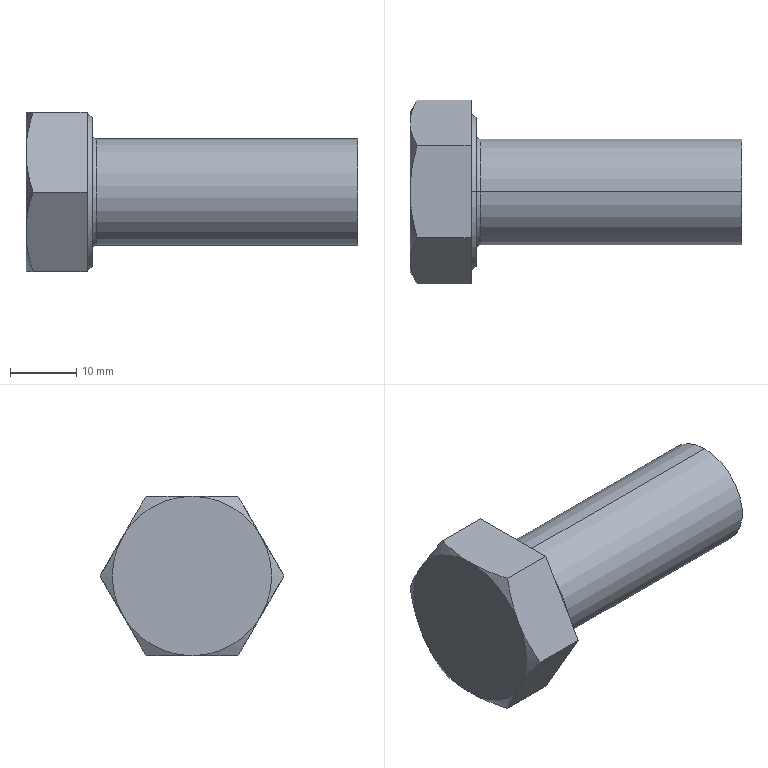Part | SolidWorks | features RevCut 3, Extrusion 1, Fillet 1, LPattern 1, Revolution 1 | 1 solid | 22 faces | box 50 x 27.713 x 24 mm | volume 12952 mm3 | plane 10 | cone 8 | torus 2 | cylinder 2 | commonest cylinder face diameters 16 x2
STEP:
#1=CARTESIAN_POINT('',(10.6,0.,8.));
#2=VERTEX_POINT('',#1);
#3=CARTESIAN_POINT('',(10.6,0.,-8.));
#4=VERTEX_POINT('',#3);
#5=CARTESIAN_POINT('',(10.6,0.,0.));
#6=DIRECTION('',(1.,0.,0.));
#7=DIRECTION('',(0.,0.,-1.));
#8=AXIS2_PLACEMENT_3D('',#5,#6,#7);
#9=CIRCLE('',#8,8.);
#10=EDGE_CURVE('',#2,#4,#9,.T.);
#11=ORIENTED_EDGE('',*,*,#10,.F.);
#12=CARTESIAN_POINT('',(10.,0.,8.6));
#13=VERTEX_POINT('',#12);
#14=CARTESIAN_POINT('',(10.6,0.,8.6));
#15=DIRECTION('',(0.,1.,0.));
#16=DIRECTION('',(0.,0.,1.));
#17=AXIS2_PLACEMENT_3D('',#14,#15,#16);
#18=CIRCLE('',#17,0.6);
#19=EDGE_CURVE('',#2,#13,#18,.T.);
#20=ORIENTED_EDGE('',*,*,#19,.T.);
#21=CARTESIAN_POINT('',(10.,0.,-8.6));
#22=VERTEX_POINT('',#21);
#23=CARTESIAN_POINT('',(10.,0.,0.));
#24=DIRECTION('',(-1.,0.,0.));
#25=DIRECTION('',(0.,0.,-1.));
#26=AXIS2_PLACEMENT_3D('',#23,#24,#25);
#27=CIRCLE('',#26,8.6);
#28=EDGE_CURVE('',#22,#13,#27,.T.);
#29=ORIENTED_EDGE('',*,*,#28,.F.);
#30=CARTESIAN_POINT('',(10.6,0.,-8.6));
#31=DIRECTION('',(0.,-1.,0.));
#32=DIRECTION('',(0.,0.,-1.));
#33=AXIS2_PLACEMENT_3D('',#30,#31,#32);
#34=CIRCLE('',#33,0.6);
#35=EDGE_CURVE('',#4,#22,#34,.T.);
#36=ORIENTED_EDGE('',*,*,#35,.F.);
#37=EDGE_LOOP('',(#11,#20,#29,#36));
#38=FACE_OUTER_BOUND('',#37,.T.);
#39=CARTESIAN_POINT('',(10.6,0.,0.));
#40=DIRECTION('',(1.,0.,0.));
#41=DIRECTION('',(0.,0.,-1.));
#42=AXIS2_PLACEMENT_3D('',#39,#40,#41);
#43=TOROIDAL_SURFACE('',#42,8.6,0.6);
#44=ADVANCED_FACE('',(#38),#43,.F.);
#45=CARTESIAN_POINT('',(50.,0.,8.));
#46=VERTEX_POINT('',#45);
#47=CARTESIAN_POINT('',(50.,0.,-8.));
#48=VERTEX_POINT('',#47);
#49=CARTESIAN_POINT('',(50.,0.,0.));
#50=DIRECTION('',(-1.,0.,0.));
#51=DIRECTION('',(0.,0.,1.));
#52=AXIS2_PLACEMENT_3D('',#49,#50,#51);
#53=CIRCLE('',#52,8.);
#54=EDGE_CURVE('',#46,#48,#53,.T.);
#55=ORIENTED_EDGE('',*,*,#54,.T.);
#56=CARTESIAN_POINT('',(0.,0.,-8.));
#57=DIRECTION('',(-1.,0.,0.));
#58=VECTOR('',#57,1000.);
#59=LINE('',#56,#58);
#60=EDGE_CURVE('',#48,#4,#59,.T.);
#61=ORIENTED_EDGE('',*,*,#60,.T.);
#62=CARTESIAN_POINT('',(10.6,0.,0.));
#63=DIRECTION('',(1.,0.,0.));
#64=DIRECTION('',(0.,0.,-1.));
#65=AXIS2_PLACEMENT_3D('',#62,#63,#64);
#66=CIRCLE('',#65,8.);
#67=EDGE_CURVE('',#4,#2,#66,.T.);
#68=ORIENTED_EDGE('',*,*,#67,.T.);
#69=CARTESIAN_POINT('',(0.,0.,8.));
#70=DIRECTION('',(-1.,0.,0.));
#71=VECTOR('',#70,1000.);
#72=LINE('',#69,#71);
#73=EDGE_CURVE('',#46,#2,#72,.T.);
#74=ORIENTED_EDGE('',*,*,#73,.F.);
#75=EDGE_LOOP('',(#55,#61,#68,#74));
#76=FACE_OUTER_BOUND('',#75,.T.);
#77=CARTESIAN_POINT('',(0.,0.,0.));
#78=DIRECTION('',(-1.,0.,0.));
#79=DIRECTION('',(0.,0.,1.));
#80=AXIS2_PLACEMENT_3D('',#77,#78,#79);
#81=CYLINDRICAL_SURFACE('',#80,8.);
#82=ADVANCED_FACE('',(#76),#81,.T.);
#83=CARTESIAN_POINT('',(10.,0.,11.245));
#84=VERTEX_POINT('',#83);
#85=CARTESIAN_POINT('',(10.,0.,-11.245));
#86=VERTEX_POINT('',#85);
#87=CARTESIAN_POINT('',(10.,0.,0.));
#88=DIRECTION('',(-1.,0.,0.));
#89=DIRECTION('',(0.,0.,1.));
#90=AXIS2_PLACEMENT_3D('',#87,#88,#89);
#91=CIRCLE('',#90,11.245);
#92=EDGE_CURVE('',#84,#86,#91,.T.);
#93=ORIENTED_EDGE('',*,*,#92,.T.);
#94=CARTESIAN_POINT('',(9.2,0.,-11.707));
#95=VERTEX_POINT('',#94);
#96=CARTESIAN_POINT('',(9.2,0.,-11.707));
#97=DIRECTION('',(-0.866,0.,-0.5));
#98=VECTOR('',#97,1000.);
#99=LINE('',#96,#98);
#100=EDGE_CURVE('',#86,#95,#99,.T.);
#101=ORIENTED_EDGE('',*,*,#100,.T.);
#102=CARTESIAN_POINT('',(9.2,0.,11.707));
#103=VERTEX_POINT('',#102);
#104=CARTESIAN_POINT('',(9.2,0.,0.));
#105=DIRECTION('',(-1.,0.,0.));
#106=DIRECTION('',(0.,0.,1.));
#107=AXIS2_PLACEMENT_3D('',#104,#105,#106);
#108=CIRCLE('',#107,11.707);
#109=EDGE_CURVE('',#103,#95,#108,.T.);
#110=ORIENTED_EDGE('',*,*,#109,.F.);
#111=CARTESIAN_POINT('',(9.2,0.,11.707));
#112=DIRECTION('',(-0.866,0.,0.5));
#113=VECTOR('',#112,1000.);
#114=LINE('',#111,#113);
#115=EDGE_CURVE('',#84,#103,#114,.T.);
#116=ORIENTED_EDGE('',*,*,#115,.F.);
#117=EDGE_LOOP('',(#93,#101,#110,#116));
#118=FACE_OUTER_BOUND('',#117,.T.);
#119=CARTESIAN_POINT('',(9.2,0.,0.));
#120=DIRECTION('',(-1.,0.,0.));
#121=DIRECTION('',(0.,0.,1.));
#122=AXIS2_PLACEMENT_3D('',#119,#120,#121);
#123=CONICAL_SURFACE('',#122,11.707,0.5236);
#124=ADVANCED_FACE('',(#118),#123,.T.);
#125=CARTESIAN_POINT('',(9.2,6.928,-12.));
#126=VERTEX_POINT('',#125);
#127=CARTESIAN_POINT('',(9.2,13.856,0.));
#128=VERTEX_POINT('',#127);
#129=CARTESIAN_POINT('',(9.2,6.928,-12.));
#130=DIRECTION('',(0.,0.5,0.866));
#131=VECTOR('',#130,1000.);
#132=LINE('',#129,#131);
#133=EDGE_CURVE('',#126,#128,#132,.T.);
#134=ORIENTED_EDGE('',*,*,#133,.F.);
#135=CARTESIAN_POINT('',(1.072,6.928,-12.));
#136=VERTEX_POINT('',#135);
#137=CARTESIAN_POINT('',(10.,6.928,-12.));
#138=DIRECTION('',(-1.,0.,0.));
#139=VECTOR('',#138,1000.);
#140=LINE('',#137,#139);
#141=EDGE_CURVE('',#126,#136,#140,.T.);
#142=ORIENTED_EDGE('',*,*,#141,.T.);
#143=CARTESIAN_POINT('',(0.,10.392,-6.));
#144=VERTEX_POINT('',#143);
#145=CARTESIAN_POINT('',(0.,10.392,-6.));
#146=CARTESIAN_POINT('',(0.,10.098,-6.509));
#147=CARTESIAN_POINT('',(0.02533,9.803,-7.021));
#148=CARTESIAN_POINT('',(0.1234,9.219,-8.033));
#149=CARTESIAN_POINT('',(0.196,8.929,-8.535));
#150=CARTESIAN_POINT('',(0.476,8.063,-10.034));
#151=CARTESIAN_POINT('',(0.7454,7.493,-11.021));
#152=CARTESIAN_POINT('',(1.072,6.928,-12.));
#153=B_SPLINE_CURVE_WITH_KNOTS('',3,(#145,#146,#147,#148,#149,#150,#151,#152),.UNSPECIFIED.,.F.,.F.,(4,2,2,4),(0.00701,0.008756,0.0105,0.01399),.UNSPECIFIED.);
#154=EDGE_CURVE('',#144,#136,#153,.T.);
#155=ORIENTED_EDGE('',*,*,#154,.F.);
#156=CARTESIAN_POINT('',(1.072,13.856,0.));
#157=VERTEX_POINT('',#156);
#158=CARTESIAN_POINT('',(1.072,13.856,0.));
#159=CARTESIAN_POINT('',(0.7446,13.29,-0.9815));
#160=CARTESIAN_POINT('',(0.4751,12.719,-1.97));
#161=CARTESIAN_POINT('',(0.1021,11.565,-3.968));
#162=CARTESIAN_POINT('',(0.,10.982,-4.978));
#163=CARTESIAN_POINT('',(0.,10.392,-6.));
#164=B_SPLINE_CURVE_WITH_KNOTS('',3,(#158,#159,#160,#161,#162,#163),.UNSPECIFIED.,.F.,.F.,(4,2,4),(0.000000238,0.003505,0.00701),.UNSPECIFIED.);
#165=EDGE_CURVE('',#157,#144,#164,.T.);
#166=ORIENTED_EDGE('',*,*,#165,.F.);
#167=CARTESIAN_POINT('',(10.,13.856,0.));
#168=DIRECTION('',(-1.,0.,0.));
#169=VECTOR('',#168,1000.);
#170=LINE('',#167,#169);
#171=EDGE_CURVE('',#128,#157,#170,.T.);
#172=ORIENTED_EDGE('',*,*,#171,.F.);
#173=EDGE_LOOP('',(#134,#142,#155,#166,#172));
#174=FACE_OUTER_BOUND('',#173,.T.);
#175=CARTESIAN_POINT('',(10.,6.928,-12.));
#176=DIRECTION('',(0.,-0.866,0.5));
#177=DIRECTION('',(0.,-0.5,-0.866));
#178=AXIS2_PLACEMENT_3D('',#175,#176,#177);
#179=PLANE('',#178);
#180=ADVANCED_FACE('',(#174),#179,.F.);
#181=CARTESIAN_POINT('',(9.2,6.928,12.));
#182=VERTEX_POINT('',#181);
#183=CARTESIAN_POINT('',(9.2,13.856,0.));
#184=DIRECTION('',(0.,-0.5,0.866));
#185=VECTOR('',#184,1000.);
#186=LINE('',#183,#185);
#187=EDGE_CURVE('',#128,#182,#186,.T.);
#188=ORIENTED_EDGE('',*,*,#187,.F.);
#189=ORIENTED_EDGE('',*,*,#171,.T.);
#190=CARTESIAN_POINT('',(0.,10.392,6.));
#191=VERTEX_POINT('',#190);
#192=CARTESIAN_POINT('',(0.,10.392,6.));
#193=CARTESIAN_POINT('',(0.,10.686,5.491));
#194=CARTESIAN_POINT('',(0.02533,10.982,4.979));
#195=CARTESIAN_POINT('',(0.1234,11.566,3.967));
#196=CARTESIAN_POINT('',(0.196,11.856,3.465));
#197=CARTESIAN_POINT('',(0.476,12.721,1.966));
#198=CARTESIAN_POINT('',(0.7454,13.291,0.9791));
#199=CARTESIAN_POINT('',(1.072,13.856,0.));
#200=B_SPLINE_CURVE_WITH_KNOTS('',3,(#192,#193,#194,#195,#196,#197,#198,#199),.UNSPECIFIED.,.F.,.F.,(4,2,2,4),(0.00701,0.008756,0.0105,0.01399),.UNSPECIFIED.);
#201=EDGE_CURVE('',#191,#157,#200,.T.);
#202=ORIENTED_EDGE('',*,*,#201,.F.);
#203=CARTESIAN_POINT('',(1.072,6.928,12.));
#204=VERTEX_POINT('',#203);
#205=CARTESIAN_POINT('',(1.072,6.928,12.));
#206=CARTESIAN_POINT('',(0.7446,7.495,11.018));
#207=CARTESIAN_POINT('',(0.4751,8.066,10.03));
#208=CARTESIAN_POINT('',(0.1021,9.219,8.032));
#209=CARTESIAN_POINT('',(0.,9.802,7.022));
#210=CARTESIAN_POINT('',(0.,10.392,6.));
#211=B_SPLINE_CURVE_WITH_KNOTS('',3,(#205,#206,#207,#208,#209,#210),.UNSPECIFIED.,.F.,.F.,(4,2,4),(0.000000238,0.003505,0.00701),.UNSPECIFIED.);
#212=EDGE_CURVE('',#204,#191,#211,.T.);
#213=ORIENTED_EDGE('',*,*,#212,.F.);
#214=CARTESIAN_POINT('',(10.,6.928,12.));
#215=DIRECTION('',(-1.,0.,0.));
#216=VECTOR('',#215,1000.);
#217=LINE('',#214,#216);
#218=EDGE_CURVE('',#182,#204,#217,.T.);
#219=ORIENTED_EDGE('',*,*,#218,.F.);
#220=EDGE_LOOP('',(#188,#189,#202,#213,#219));
#221=FACE_OUTER_BOUND('',#220,.T.);
#222=CARTESIAN_POINT('',(10.,13.856,0.));
#223=DIRECTION('',(0.,-0.866,-0.5));
#224=DIRECTION('',(0.,0.5,-0.866));
#225=AXIS2_PLACEMENT_3D('',#222,#223,#224);
#226=PLANE('',#225);
#227=ADVANCED_FACE('',(#221),#226,.F.);
#228=CARTESIAN_POINT('',(9.2,-6.928,12.));
#229=VERTEX_POINT('',#228);
#230=CARTESIAN_POINT('',(9.2,6.928,12.));
#231=DIRECTION('',(0.,-1.,0.));
#232=VECTOR('',#231,1000.);
#233=LINE('',#230,#232);
#234=EDGE_CURVE('',#182,#229,#233,.T.);
#235=ORIENTED_EDGE('',*,*,#234,.F.);
#236=ORIENTED_EDGE('',*,*,#218,.T.);
#237=CARTESIAN_POINT('',(0.,0.,12.));
#238=VERTEX_POINT('',#237);
#239=CARTESIAN_POINT('',(0.,0.,12.));
#240=CARTESIAN_POINT('',(0.,0.5865,12.));
#241=CARTESIAN_POINT('',(0.02506,1.176,12.));
#242=CARTESIAN_POINT('',(0.1242,2.355,12.));
#243=CARTESIAN_POINT('',(0.1975,2.939,12.));
#244=CARTESIAN_POINT('',(0.4791,4.673,12.));
#245=CARTESIAN_POINT('',(0.7483,5.808,12.));
#246=CARTESIAN_POINT('',(1.072,6.928,12.));
#247=B_SPLINE_CURVE_WITH_KNOTS('',3,(#239,#240,#241,#242,#243,#244,#245,#246),.UNSPECIFIED.,.F.,.F.,(4,2,2,4),(0.01982,0.02158,0.02333,0.02684),.UNSPECIFIED.);
#248=EDGE_CURVE('',#238,#204,#247,.T.);
#249=ORIENTED_EDGE('',*,*,#248,.F.);
#250=CARTESIAN_POINT('',(1.072,-6.928,12.));
#251=VERTEX_POINT('',#250);
#252=CARTESIAN_POINT('',(1.072,-6.928,12.));
#253=CARTESIAN_POINT('',(0.7461,-5.8,12.));
#254=CARTESIAN_POINT('',(0.4736,-4.647,12.));
#255=CARTESIAN_POINT('',(0.1008,-2.335,12.));
#256=CARTESIAN_POINT('',(0.,-1.172,12.));
#257=CARTESIAN_POINT('',(0.,0.,12.));
#258=B_SPLINE_CURVE_WITH_KNOTS('',3,(#252,#253,#254,#255,#256,#257),.UNSPECIFIED.,.F.,.F.,(4,2,4),(0.01281,0.01632,0.01982),.UNSPECIFIED.);
#259=EDGE_CURVE('',#251,#238,#258,.T.);
#260=ORIENTED_EDGE('',*,*,#259,.F.);
#261=CARTESIAN_POINT('',(10.,-6.928,12.));
#262=DIRECTION('',(-1.,0.,0.));
#263=VECTOR('',#262,1000.);
#264=LINE('',#261,#263);
#265=EDGE_CURVE('',#229,#251,#264,.T.);
#266=ORIENTED_EDGE('',*,*,#265,.F.);
#267=EDGE_LOOP('',(#235,#236,#249,#260,#266));
#268=FACE_OUTER_BOUND('',#267,.T.);
#269=CARTESIAN_POINT('',(10.,6.928,12.));
#270=DIRECTION('',(0.,0.,-1.));
#271=DIRECTION('',(-1.,0.,0.));
#272=AXIS2_PLACEMENT_3D('',#269,#270,#271);
#273=PLANE('',#272);
#274=ADVANCED_FACE('',(#268),#273,.F.);
#275=CARTESIAN_POINT('',(9.2,-13.856,0.));
#276=VERTEX_POINT('',#275);
#277=CARTESIAN_POINT('',(9.2,-13.856,0.));
#278=DIRECTION('',(0.,-0.5,-0.866));
#279=VECTOR('',#278,1000.);
#280=LINE('',#277,#279);
#281=EDGE_CURVE('',#229,#276,#280,.T.);
#282=ORIENTED_EDGE('',*,*,#281,.F.);
#283=ORIENTED_EDGE('',*,*,#265,.T.);
#284=CARTESIAN_POINT('',(0.,-10.392,6.));
#285=VERTEX_POINT('',#284);
#286=CARTESIAN_POINT('',(0.,-10.392,6.));
#287=CARTESIAN_POINT('',(0.,-10.098,6.509));
#288=CARTESIAN_POINT('',(0.02533,-9.803,7.021));
#289=CARTESIAN_POINT('',(0.1234,-9.219,8.033));
#290=CARTESIAN_POINT('',(0.196,-8.929,8.535));
#291=CARTESIAN_POINT('',(0.476,-8.063,10.034));
#292=CARTESIAN_POINT('',(0.7454,-7.493,11.021));
#293=CARTESIAN_POINT('',(1.072,-6.928,12.));
#294=B_SPLINE_CURVE_WITH_KNOTS('',3,(#286,#287,#288,#289,#290,#291,#292,#293),.UNSPECIFIED.,.F.,.F.,(4,2,2,4),(0.00701,0.008756,0.0105,0.01399),.UNSPECIFIED.);
#295=EDGE_CURVE('',#285,#251,#294,.T.);
#296=ORIENTED_EDGE('',*,*,#295,.F.);
#297=CARTESIAN_POINT('',(1.072,-13.856,0.));
#298=VERTEX_POINT('',#297);
#299=CARTESIAN_POINT('',(1.072,-13.856,0.));
#300=CARTESIAN_POINT('',(0.7446,-13.29,0.9815));
#301=CARTESIAN_POINT('',(0.4751,-12.719,1.97));
#302=CARTESIAN_POINT('',(0.1021,-11.565,3.968));
#303=CARTESIAN_POINT('',(0.,-10.982,4.978));
#304=CARTESIAN_POINT('',(0.,-10.392,6.));
#305=B_SPLINE_CURVE_WITH_KNOTS('',3,(#299,#300,#301,#302,#303,#304),.UNSPECIFIED.,.F.,.F.,(4,2,4),(0.000000238,0.003505,0.00701),.UNSPECIFIED.);
#306=EDGE_CURVE('',#298,#285,#305,.T.);
#307=ORIENTED_EDGE('',*,*,#306,.F.);
#308=CARTESIAN_POINT('',(10.,-13.856,0.));
#309=DIRECTION('',(-1.,0.,0.));
#310=VECTOR('',#309,1000.);
#311=LINE('',#308,#310);
#312=EDGE_CURVE('',#276,#298,#311,.T.);
#313=ORIENTED_EDGE('',*,*,#312,.F.);
#314=EDGE_LOOP('',(#282,#283,#296,#307,#313));
#315=FACE_OUTER_BOUND('',#314,.T.);
#316=CARTESIAN_POINT('',(10.,-13.856,0.));
#317=DIRECTION('',(0.,0.866,-0.5));
#318=DIRECTION('',(0.,0.5,0.866));
#319=AXIS2_PLACEMENT_3D('',#316,#317,#318);
#320=PLANE('',#319);
#321=ADVANCED_FACE('',(#315),#320,.F.);
#322=CARTESIAN_POINT('',(9.2,-6.928,-12.));
#323=VERTEX_POINT('',#322);
#324=CARTESIAN_POINT('',(9.2,-6.928,-12.));
#325=DIRECTION('',(0.,0.5,-0.866));
#326=VECTOR('',#325,1000.);
#327=LINE('',#324,#326);
#328=EDGE_CURVE('',#276,#323,#327,.T.);
#329=ORIENTED_EDGE('',*,*,#328,.F.);
#330=ORIENTED_EDGE('',*,*,#312,.T.);
#331=CARTESIAN_POINT('',(0.,-10.392,-6.));
#332=VERTEX_POINT('',#331);
#333=CARTESIAN_POINT('',(0.,-10.392,-6.));
#334=CARTESIAN_POINT('',(0.,-10.686,-5.491));
#335=CARTESIAN_POINT('',(0.02533,-10.982,-4.979));
#336=CARTESIAN_POINT('',(0.1234,-11.566,-3.967));
#337=CARTESIAN_POINT('',(0.196,-11.856,-3.465));
#338=CARTESIAN_POINT('',(0.476,-12.721,-1.966));
#339=CARTESIAN_POINT('',(0.7454,-13.291,-0.9791));
#340=CARTESIAN_POINT('',(1.072,-13.856,0.));
#341=B_SPLINE_CURVE_WITH_KNOTS('',3,(#333,#334,#335,#336,#337,#338,#339,#340),.UNSPECIFIED.,.F.,.F.,(4,2,2,4),(0.00701,0.008756,0.0105,0.01399),.UNSPECIFIED.);
#342=EDGE_CURVE('',#332,#298,#341,.T.);
#343=ORIENTED_EDGE('',*,*,#342,.F.);
#344=CARTESIAN_POINT('',(1.072,-6.928,-12.));
#345=VERTEX_POINT('',#344);
#346=CARTESIAN_POINT('',(1.072,-6.928,-12.));
#347=CARTESIAN_POINT('',(0.7446,-7.495,-11.018));
#348=CARTESIAN_POINT('',(0.4751,-8.066,-10.03));
#349=CARTESIAN_POINT('',(0.1021,-9.219,-8.032));
#350=CARTESIAN_POINT('',(0.,-9.802,-7.022));
#351=CARTESIAN_POINT('',(0.,-10.392,-6.));
#352=B_SPLINE_CURVE_WITH_KNOTS('',3,(#346,#347,#348,#349,#350,#351),.UNSPECIFIED.,.F.,.F.,(4,2,4),(0.000000238,0.003505,0.00701),.UNSPECIFIED.);
#353=EDGE_CURVE('',#345,#332,#352,.T.);
#354=ORIENTED_EDGE('',*,*,#353,.F.);
#355=CARTESIAN_POINT('',(10.,-6.928,-12.));
#356=DIRECTION('',(-1.,0.,0.));
#357=VECTOR('',#356,1000.);
#358=LINE('',#355,#357);
#359=EDGE_CURVE('',#323,#345,#358,.T.);
#360=ORIENTED_EDGE('',*,*,#359,.F.);
#361=EDGE_LOOP('',(#329,#330,#343,#354,#360));
#362=FACE_OUTER_BOUND('',#361,.T.);
#363=CARTESIAN_POINT('',(10.,-6.928,-12.));
#364=DIRECTION('',(0.,0.866,0.5));
#365=DIRECTION('',(0.,-0.5,0.866));
#366=AXIS2_PLACEMENT_3D('',#363,#364,#365);
#367=PLANE('',#366);
#368=ADVANCED_FACE('',(#362),#367,.F.);
#369=CARTESIAN_POINT('',(9.2,6.928,-12.));
#370=DIRECTION('',(0.,1.,0.));
#371=VECTOR('',#370,1000.);
#372=LINE('',#369,#371);
#373=EDGE_CURVE('',#323,#126,#372,.T.);
#374=ORIENTED_EDGE('',*,*,#373,.F.);
#375=ORIENTED_EDGE('',*,*,#359,.T.);
#376=CARTESIAN_POINT('',(0.,0.,-12.));
#377=VERTEX_POINT('',#376);
#378=CARTESIAN_POINT('',(0.,0.,-12.));
#379=CARTESIAN_POINT('',(0.,-1.172,-12.));
#380=CARTESIAN_POINT('',(0.1008,-2.335,-12.));
#381=CARTESIAN_POINT('',(0.4736,-4.647,-12.));
#382=CARTESIAN_POINT('',(0.7461,-5.8,-12.));
#383=CARTESIAN_POINT('',(1.072,-6.928,-12.));
#384=B_SPLINE_CURVE_WITH_KNOTS('',3,(#378,#379,#380,#381,#382,#383),.UNSPECIFIED.,.F.,.F.,(4,2,4),(0.03938,0.04289,0.0464),.UNSPECIFIED.);
#385=EDGE_CURVE('',#377,#345,#384,.T.);
#386=ORIENTED_EDGE('',*,*,#385,.F.);
#387=CARTESIAN_POINT('',(1.072,6.928,-12.));
#388=CARTESIAN_POINT('',(0.7483,5.808,-12.));
#389=CARTESIAN_POINT('',(0.4791,4.673,-12.));
#390=CARTESIAN_POINT('',(0.1975,2.939,-12.));
#391=CARTESIAN_POINT('',(0.1242,2.355,-12.));
#392=CARTESIAN_POINT('',(0.02506,1.176,-12.));
#393=CARTESIAN_POINT('',(0.,0.5865,-12.));
#394=CARTESIAN_POINT('',(0.,0.,-12.));
#395=B_SPLINE_CURVE_WITH_KNOTS('',3,(#387,#388,#389,#390,#391,#392,#393,#394),.UNSPECIFIED.,.F.,.F.,(4,2,2,4),(0.03236,0.03587,0.03763,0.03938),.UNSPECIFIED.);
#396=EDGE_CURVE('',#136,#377,#395,.T.);
#397=ORIENTED_EDGE('',*,*,#396,.F.);
#398=ORIENTED_EDGE('',*,*,#141,.F.);
#399=EDGE_LOOP('',(#374,#375,#386,#397,#398));
#400=FACE_OUTER_BOUND('',#399,.T.);
#401=CARTESIAN_POINT('',(10.,6.928,-12.));
#402=DIRECTION('',(0.,0.,1.));
#403=DIRECTION('',(0.,-1.,0.));
#404=AXIS2_PLACEMENT_3D('',#401,#402,#403);
#405=PLANE('',#404);
#406=ADVANCED_FACE('',(#400),#405,.F.);
#407=ORIENTED_EDGE('',*,*,#353,.T.);
#408=CARTESIAN_POINT('',(0.,0.,0.));
#409=DIRECTION('',(1.,0.,0.));
#410=DIRECTION('',(0.,0.,-1.));
#411=AXIS2_PLACEMENT_3D('',#408,#409,#410);
#412=CIRCLE('',#411,12.);
#413=EDGE_CURVE('',#332,#377,#412,.T.);
#414=ORIENTED_EDGE('',*,*,#413,.T.);
#415=ORIENTED_EDGE('',*,*,#385,.T.);
#416=EDGE_LOOP('',(#407,#414,#415));
#417=FACE_OUTER_BOUND('',#416,.T.);
#418=CARTESIAN_POINT('',(0.,0.,0.));
#419=DIRECTION('',(1.,0.,0.));
#420=DIRECTION('',(0.,0.,-1.));
#421=AXIS2_PLACEMENT_3D('',#418,#419,#420);
#422=CONICAL_SURFACE('',#421,12.,1.047);
#423=ADVANCED_FACE('',(#417),#422,.T.);
#424=ORIENTED_EDGE('',*,*,#306,.T.);
#425=CARTESIAN_POINT('',(0.,0.,0.));
#426=DIRECTION('',(1.,0.,0.));
#427=DIRECTION('',(0.,0.,-1.));
#428=AXIS2_PLACEMENT_3D('',#425,#426,#427);
#429=CIRCLE('',#428,12.);
#430=EDGE_CURVE('',#285,#332,#429,.T.);
#431=ORIENTED_EDGE('',*,*,#430,.T.);
#432=ORIENTED_EDGE('',*,*,#342,.T.);
#433=EDGE_LOOP('',(#424,#431,#432));
#434=FACE_OUTER_BOUND('',#433,.T.);
#435=CARTESIAN_POINT('',(0.,0.,0.));
#436=DIRECTION('',(1.,0.,0.));
#437=DIRECTION('',(0.,0.,-1.));
#438=AXIS2_PLACEMENT_3D('',#435,#436,#437);
#439=CONICAL_SURFACE('',#438,12.,1.047);
#440=ADVANCED_FACE('',(#434),#439,.T.);
#441=ORIENTED_EDGE('',*,*,#259,.T.);
#442=CARTESIAN_POINT('',(0.,0.,0.));
#443=DIRECTION('',(1.,0.,0.));
#444=DIRECTION('',(0.,0.,-1.));
#445=AXIS2_PLACEMENT_3D('',#442,#443,#444);
#446=CIRCLE('',#445,12.);
#447=EDGE_CURVE('',#238,#285,#446,.T.);
#448=ORIENTED_EDGE('',*,*,#447,.T.);
#449=ORIENTED_EDGE('',*,*,#295,.T.);
#450=EDGE_LOOP('',(#441,#448,#449));
#451=FACE_OUTER_BOUND('',#450,.T.);
#452=CARTESIAN_POINT('',(0.,0.,0.));
#453=DIRECTION('',(1.,0.,0.));
#454=DIRECTION('',(0.,0.,-1.));
#455=AXIS2_PLACEMENT_3D('',#452,#453,#454);
#456=CONICAL_SURFACE('',#455,12.,1.047);
#457=ADVANCED_FACE('',(#451),#456,.T.);
#458=ORIENTED_EDGE('',*,*,#248,.T.);
#459=ORIENTED_EDGE('',*,*,#212,.T.);
#460=CARTESIAN_POINT('',(0.,0.,0.));
#461=DIRECTION('',(-1.,0.,0.));
#462=DIRECTION('',(0.,0.,1.));
#463=AXIS2_PLACEMENT_3D('',#460,#461,#462);
#464=CIRCLE('',#463,12.);
#465=EDGE_CURVE('',#238,#191,#464,.T.);
#466=ORIENTED_EDGE('',*,*,#465,.F.);
#467=EDGE_LOOP('',(#458,#459,#466));
#468=FACE_OUTER_BOUND('',#467,.T.);
#469=CARTESIAN_POINT('',(0.,0.,0.));
#470=DIRECTION('',(1.,0.,0.));
#471=DIRECTION('',(0.,0.,-1.));
#472=AXIS2_PLACEMENT_3D('',#469,#470,#471);
#473=CONICAL_SURFACE('',#472,12.,1.047);
#474=ADVANCED_FACE('',(#468),#473,.T.);
#475=ORIENTED_EDGE('',*,*,#201,.T.);
#476=ORIENTED_EDGE('',*,*,#165,.T.);
#477=CARTESIAN_POINT('',(0.,0.,0.));
#478=DIRECTION('',(1.,0.,0.));
#479=DIRECTION('',(0.,0.,-1.));
#480=AXIS2_PLACEMENT_3D('',#477,#478,#479);
#481=CIRCLE('',#480,12.);
#482=EDGE_CURVE('',#144,#191,#481,.T.);
#483=ORIENTED_EDGE('',*,*,#482,.T.);
#484=EDGE_LOOP('',(#475,#476,#483));
#485=FACE_OUTER_BOUND('',#484,.T.);
#486=CARTESIAN_POINT('',(0.,0.,0.));
#487=DIRECTION('',(1.,0.,0.));
#488=DIRECTION('',(0.,0.,-1.));
#489=AXIS2_PLACEMENT_3D('',#486,#487,#488);
#490=CONICAL_SURFACE('',#489,12.,1.047);
#491=ADVANCED_FACE('',(#485),#490,.T.);
#492=ORIENTED_EDGE('',*,*,#154,.T.);
#493=ORIENTED_EDGE('',*,*,#396,.T.);
#494=CARTESIAN_POINT('',(0.,0.,0.));
#495=DIRECTION('',(1.,0.,0.));
#496=DIRECTION('',(0.,0.,-1.));
#497=AXIS2_PLACEMENT_3D('',#494,#495,#496);
#498=CIRCLE('',#497,12.);
#499=EDGE_CURVE('',#377,#144,#498,.T.);
#500=ORIENTED_EDGE('',*,*,#499,.T.);
#501=EDGE_LOOP('',(#492,#493,#500));
#502=FACE_OUTER_BOUND('',#501,.T.);
#503=CARTESIAN_POINT('',(0.,0.,0.));
#504=DIRECTION('',(1.,0.,0.));
#505=DIRECTION('',(0.,0.,-1.));
#506=AXIS2_PLACEMENT_3D('',#503,#504,#505);
#507=CONICAL_SURFACE('',#506,12.,1.047);
#508=ADVANCED_FACE('',(#502),#507,.T.);
#509=ORIENTED_EDGE('',*,*,#499,.F.);
#510=ORIENTED_EDGE('',*,*,#413,.F.);
#511=ORIENTED_EDGE('',*,*,#430,.F.);
#512=ORIENTED_EDGE('',*,*,#447,.F.);
#513=ORIENTED_EDGE('',*,*,#465,.T.);
#514=ORIENTED_EDGE('',*,*,#482,.F.);
#515=EDGE_LOOP('',(#509,#510,#511,#512,#513,#514));
#516=FACE_OUTER_BOUND('',#515,.T.);
#517=CARTESIAN_POINT('',(0.,13.856,0.));
#518=DIRECTION('',(1.,0.,0.));
#519=DIRECTION('',(0.,0.,-1.));
#520=AXIS2_PLACEMENT_3D('',#517,#518,#519);
#521=PLANE('',#520);
#522=ADVANCED_FACE('',(#516),#521,.F.);
#523=ORIENTED_EDGE('',*,*,#109,.T.);
#524=CARTESIAN_POINT('',(9.2,0.,0.));
#525=DIRECTION('',(-1.,0.,0.));
#526=DIRECTION('',(0.,0.,1.));
#527=AXIS2_PLACEMENT_3D('',#524,#525,#526);
#528=CIRCLE('',#527,11.707);
#529=EDGE_CURVE('',#95,#103,#528,.T.);
#530=ORIENTED_EDGE('',*,*,#529,.T.);
#531=EDGE_LOOP('',(#523,#530));
#532=FACE_BOUND('',#531,.T.);
#533=ORIENTED_EDGE('',*,*,#133,.T.);
#534=ORIENTED_EDGE('',*,*,#187,.T.);
#535=ORIENTED_EDGE('',*,*,#234,.T.);
#536=ORIENTED_EDGE('',*,*,#281,.T.);
#537=ORIENTED_EDGE('',*,*,#328,.T.);
#538=ORIENTED_EDGE('',*,*,#373,.T.);
#539=EDGE_LOOP('',(#533,#534,#535,#536,#537,#538));
#540=FACE_OUTER_BOUND('',#539,.T.);
#541=CARTESIAN_POINT('',(9.2,11.707,0.));
#542=DIRECTION('',(1.,0.,0.));
#543=DIRECTION('',(0.,0.,-1.));
#544=AXIS2_PLACEMENT_3D('',#541,#542,#543);
#545=PLANE('',#544);
#546=ADVANCED_FACE('',(#532,#540),#545,.T.);
#547=ORIENTED_EDGE('',*,*,#100,.F.);
#548=CARTESIAN_POINT('',(10.,0.,0.));
#549=DIRECTION('',(-1.,0.,0.));
#550=DIRECTION('',(0.,0.,1.));
#551=AXIS2_PLACEMENT_3D('',#548,#549,#550);
#552=CIRCLE('',#551,11.245);
#553=EDGE_CURVE('',#86,#84,#552,.T.);
#554=ORIENTED_EDGE('',*,*,#553,.T.);
#555=ORIENTED_EDGE('',*,*,#115,.T.);
#556=ORIENTED_EDGE('',*,*,#529,.F.);
#557=EDGE_LOOP('',(#547,#554,#555,#556));
#558=FACE_OUTER_BOUND('',#557,.T.);
#559=CARTESIAN_POINT('',(9.2,0.,0.));
#560=DIRECTION('',(-1.,0.,0.));
#561=DIRECTION('',(0.,0.,1.));
#562=AXIS2_PLACEMENT_3D('',#559,#560,#561);
#563=CONICAL_SURFACE('',#562,11.707,0.5236);
#564=ADVANCED_FACE('',(#558),#563,.T.);
#565=ORIENTED_EDGE('',*,*,#54,.F.);
#566=CARTESIAN_POINT('',(50.,0.,0.));
#567=DIRECTION('',(-1.,0.,0.));
#568=DIRECTION('',(0.,0.,1.));
#569=AXIS2_PLACEMENT_3D('',#566,#567,#568);
#570=CIRCLE('',#569,8.);
#571=EDGE_CURVE('',#48,#46,#570,.T.);
#572=ORIENTED_EDGE('',*,*,#571,.F.);
#573=EDGE_LOOP('',(#565,#572));
#574=FACE_OUTER_BOUND('',#573,.T.);
#575=CARTESIAN_POINT('',(50.,0.,0.));
#576=DIRECTION('',(-1.,0.,0.));
#577=DIRECTION('',(0.,0.,1.));
#578=AXIS2_PLACEMENT_3D('',#575,#576,#577);
#579=PLANE('',#578);
#580=ADVANCED_FACE('',(#574),#579,.F.);
#581=ORIENTED_EDGE('',*,*,#60,.F.);
#582=ORIENTED_EDGE('',*,*,#571,.T.);
#583=ORIENTED_EDGE('',*,*,#73,.T.);
#584=ORIENTED_EDGE('',*,*,#10,.T.);
#585=EDGE_LOOP('',(#581,#582,#583,#584));
#586=FACE_OUTER_BOUND('',#585,.T.);
#587=CARTESIAN_POINT('',(0.,0.,0.));
#588=DIRECTION('',(-1.,0.,0.));
#589=DIRECTION('',(0.,0.,1.));
#590=AXIS2_PLACEMENT_3D('',#587,#588,#589);
#591=CYLINDRICAL_SURFACE('',#590,8.);
#592=ADVANCED_FACE('',(#586),#591,.T.);
#593=ORIENTED_EDGE('',*,*,#28,.T.);
#594=CARTESIAN_POINT('',(10.,0.,0.));
#595=DIRECTION('',(-1.,0.,0.));
#596=DIRECTION('',(0.,0.,-1.));
#597=AXIS2_PLACEMENT_3D('',#594,#595,#596);
#598=CIRCLE('',#597,8.6);
#599=EDGE_CURVE('',#13,#22,#598,.T.);
#600=ORIENTED_EDGE('',*,*,#599,.T.);
#601=EDGE_LOOP('',(#593,#600));
#602=FACE_BOUND('',#601,.T.);
#603=ORIENTED_EDGE('',*,*,#92,.F.);
#604=ORIENTED_EDGE('',*,*,#553,.F.);
#605=EDGE_LOOP('',(#603,#604));
#606=FACE_OUTER_BOUND('',#605,.T.);
#607=CARTESIAN_POINT('',(10.,13.856,0.));
#608=DIRECTION('',(1.,0.,0.));
#609=DIRECTION('',(0.,0.,-1.));
#610=AXIS2_PLACEMENT_3D('',#607,#608,#609);
#611=PLANE('',#610);
#612=ADVANCED_FACE('',(#602,#606),#611,.T.);
#613=ORIENTED_EDGE('',*,*,#19,.F.);
#614=ORIENTED_EDGE('',*,*,#67,.F.);
#615=ORIENTED_EDGE('',*,*,#35,.T.);
#616=ORIENTED_EDGE('',*,*,#599,.F.);
#617=EDGE_LOOP('',(#613,#614,#615,#616));
#618=FACE_OUTER_BOUND('',#617,.T.);
#619=CARTESIAN_POINT('',(10.6,0.,0.));
#620=DIRECTION('',(1.,0.,0.));
#621=DIRECTION('',(0.,0.,-1.));
#622=AXIS2_PLACEMENT_3D('',#619,#620,#621);
#623=TOROIDAL_SURFACE('',#622,8.6,0.6);
#624=ADVANCED_FACE('',(#618),#623,.F.);
#625=CLOSED_SHELL('',(#44,#82,#124,#180,#227,#274,#321,#368,#406,#423,#440,#457,#474,#491,#508,#522,#546,#564,#580,#592,#612,#624));
#626=MANIFOLD_SOLID_BREP('',#625);
#627=CARTESIAN_POINT('',(0.,0.,0.));
#628=DIRECTION('',(0.,0.,1.));
#629=DIRECTION('',(1.,0.,0.));
#630=AXIS2_PLACEMENT_3D('',#627,#628,#629);
#631=(LENGTH_UNIT()NAMED_UNIT(*)SI_UNIT(.MILLI.,.METRE.));
#632=UNCERTAINTY_MEASURE_WITH_UNIT(LENGTH_MEASURE(0.00001),#631,'','');
#633=(NAMED_UNIT(*)PLANE_ANGLE_UNIT()SI_UNIT($,.RADIAN.));
#634=(NAMED_UNIT(*)SI_UNIT($,.STERADIAN.)SOLID_ANGLE_UNIT());
#635=(GEOMETRIC_REPRESENTATION_CONTEXT(3)GLOBAL_UNCERTAINTY_ASSIGNED_CONTEXT((#632))GLOBAL_UNIT_ASSIGNED_CONTEXT((#631,#633,#634))REPRESENTATION_CONTEXT('',''));
#636=ADVANCED_BREP_SHAPE_REPRESENTATION('',(#626,#630),#635);